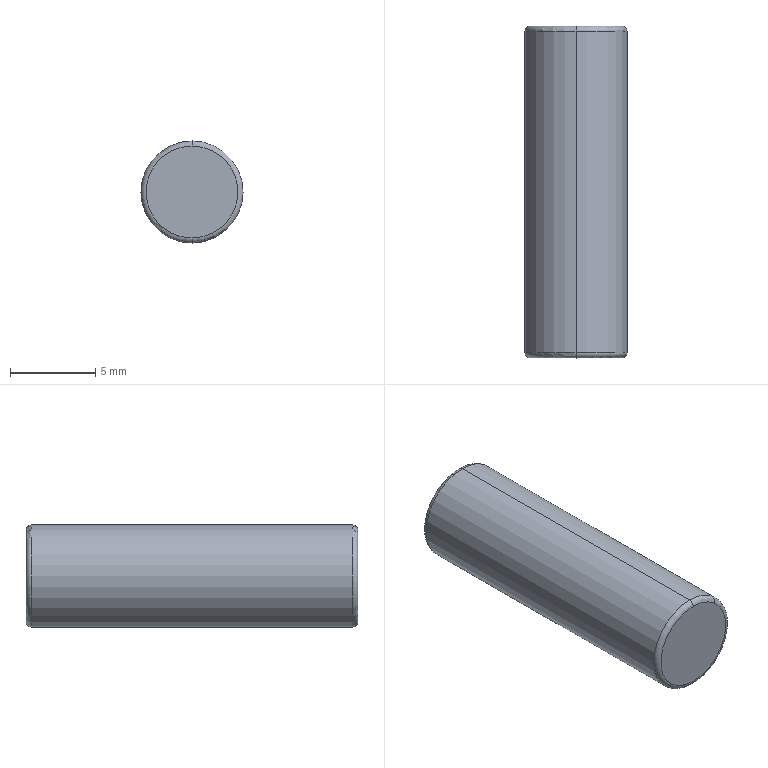Part | STEP file | 1 solid | 8 faces | box 6 x 19.5 x 6 mm | volume 550.638 mm3 | torus 4 | cylinder 2 | plane 2 | commonest cylinder face diameters 6 x2
STEP:
#1=CARTESIAN_POINT('',(0.,0.,0.));
#2=DIRECTION('',(0.,0.,1.));
#3=DIRECTION('',(1.,0.,0.));
#4=AXIS2_PLACEMENT_3D('',#1,#2,#3);
#5=CARTESIAN_POINT('',(0.,9.45,-3.));
#6=VERTEX_POINT('',#5);
#7=CARTESIAN_POINT('',(0.,9.45,3.));
#8=VERTEX_POINT('',#7);
#9=CARTESIAN_POINT('',(0.,9.45,0.));
#10=DIRECTION('',(0.,-1.,0.));
#11=DIRECTION('',(0.,0.,1.));
#12=AXIS2_PLACEMENT_3D('',#9,#10,#11);
#13=CIRCLE('',#12,3.);
#14=CARTESIAN_POINT('',(0.,9.45,0.));
#15=DIRECTION('',(0.,1.,0.));
#16=DIRECTION('',(0.,0.,1.));
#17=AXIS2_PLACEMENT_3D('',#14,#15,#16);
#18=TOROIDAL_SURFACE('',#17,2.7,0.3);
#19=CARTESIAN_POINT('',(6.283,0.));
#20=DIRECTION('',(-1.,0.));
#21=VECTOR('',#20,1.);
#22=LINE('',#19,#21);
#23=(GEOMETRIC_REPRESENTATION_CONTEXT(2)PARAMETRIC_REPRESENTATION_CONTEXT()REPRESENTATION_CONTEXT('',''));
#24=DEFINITIONAL_REPRESENTATION('',(#22),#23);
#25=PCURVE('',#18,#24);
#26=CARTESIAN_POINT('',(0.,9.75,0.));
#27=DIRECTION('',(0.,-1.,0.));
#28=DIRECTION('',(0.,0.,-1.));
#29=AXIS2_PLACEMENT_3D('',#26,#27,#28);
#30=CYLINDRICAL_SURFACE('',#29,3.);
#31=CARTESIAN_POINT('',(-3.142,0.3));
#32=DIRECTION('',(1.,0.));
#33=VECTOR('',#32,1.);
#34=LINE('',#31,#33);
#35=(GEOMETRIC_REPRESENTATION_CONTEXT(2)PARAMETRIC_REPRESENTATION_CONTEXT()REPRESENTATION_CONTEXT('',''));
#36=DEFINITIONAL_REPRESENTATION('',(#34),#35);
#37=PCURVE('',#30,#36);
#38=SURFACE_CURVE('',#13,(#25,#37),.PCURVE_S1.);
#39=EDGE_CURVE('',#6,#8,#38,.T.);
#40=ORIENTED_EDGE('',*,*,#39,.F.);
#41=CARTESIAN_POINT('',(0.,9.75,-2.7));
#42=VERTEX_POINT('',#41);
#43=CARTESIAN_POINT('',(0.,9.45,-2.7));
#44=DIRECTION('',(1.,0.,0.));
#45=DIRECTION('',(0.,0.,-1.));
#46=AXIS2_PLACEMENT_3D('',#43,#44,#45);
#47=CIRCLE('',#46,0.3);
#48=CARTESIAN_POINT('',(3.142,0.));
#49=DIRECTION('',(0.,1.));
#50=VECTOR('',#49,1.);
#51=LINE('',#48,#50);
#52=(GEOMETRIC_REPRESENTATION_CONTEXT(2)PARAMETRIC_REPRESENTATION_CONTEXT()REPRESENTATION_CONTEXT('',''));
#53=DEFINITIONAL_REPRESENTATION('',(#51),#52);
#54=PCURVE('',#18,#53);
#55=CARTESIAN_POINT('',(0.,9.45,0.));
#56=DIRECTION('',(0.,1.,0.));
#57=DIRECTION('',(0.,0.,1.));
#58=AXIS2_PLACEMENT_3D('',#55,#56,#57);
#59=TOROIDAL_SURFACE('',#58,2.7,0.3);
#60=CARTESIAN_POINT('',(3.142,0.));
#61=DIRECTION('',(0.,1.));
#62=VECTOR('',#61,1.);
#63=LINE('',#60,#62);
#64=(GEOMETRIC_REPRESENTATION_CONTEXT(2)PARAMETRIC_REPRESENTATION_CONTEXT()REPRESENTATION_CONTEXT('',''));
#65=DEFINITIONAL_REPRESENTATION('',(#63),#64);
#66=PCURVE('',#59,#65);
#67=SURFACE_CURVE('',#47,(#54,#66),.PCURVE_S1.);
#68=EDGE_CURVE('',#6,#42,#67,.T.);
#69=ORIENTED_EDGE('',*,*,#68,.T.);
#70=CARTESIAN_POINT('',(0.,9.75,2.7));
#71=VERTEX_POINT('',#70);
#72=CARTESIAN_POINT('',(0.,9.75,0.));
#73=DIRECTION('',(0.,1.,0.));
#74=DIRECTION('',(0.,0.,1.));
#75=AXIS2_PLACEMENT_3D('',#72,#73,#74);
#76=CIRCLE('',#75,2.7);
#77=CARTESIAN_POINT('',(0.,1.571));
#78=DIRECTION('',(1.,0.));
#79=VECTOR('',#78,1.);
#80=LINE('',#77,#79);
#81=(GEOMETRIC_REPRESENTATION_CONTEXT(2)PARAMETRIC_REPRESENTATION_CONTEXT()REPRESENTATION_CONTEXT('',''));
#82=DEFINITIONAL_REPRESENTATION('',(#80),#81);
#83=PCURVE('',#18,#82);
#84=CARTESIAN_POINT('',(0.,9.75,0.));
#85=DIRECTION('',(0.,1.,0.));
#86=DIRECTION('',(0.,0.,1.));
#87=AXIS2_PLACEMENT_3D('',#84,#85,#86);
#88=PLANE('',#87);
#89=CARTESIAN_POINT('',(0.,0.));
#90=DIRECTION('',(1.,0.));
#91=AXIS2_PLACEMENT_2D('',#89,#90);
#92=CIRCLE('',#91,2.7);
#93=(GEOMETRIC_REPRESENTATION_CONTEXT(2)PARAMETRIC_REPRESENTATION_CONTEXT()REPRESENTATION_CONTEXT('',''));
#94=DEFINITIONAL_REPRESENTATION('',(#92),#93);
#95=PCURVE('',#88,#94);
#96=SURFACE_CURVE('',#76,(#83,#95),.PCURVE_S1.);
#97=EDGE_CURVE('',#71,#42,#96,.T.);
#98=ORIENTED_EDGE('',*,*,#97,.F.);
#99=CARTESIAN_POINT('',(0.,9.45,2.7));
#100=DIRECTION('',(-1.,0.,0.));
#101=DIRECTION('',(0.,0.,1.));
#102=AXIS2_PLACEMENT_3D('',#99,#100,#101);
#103=CIRCLE('',#102,0.3);
#104=CARTESIAN_POINT('',(0.,0.));
#105=DIRECTION('',(0.,1.));
#106=VECTOR('',#105,1.);
#107=LINE('',#104,#106);
#108=(GEOMETRIC_REPRESENTATION_CONTEXT(2)PARAMETRIC_REPRESENTATION_CONTEXT()REPRESENTATION_CONTEXT('',''));
#109=DEFINITIONAL_REPRESENTATION('',(#107),#108);
#110=PCURVE('',#18,#109);
#111=CARTESIAN_POINT('',(6.283,0.));
#112=DIRECTION('',(0.,1.));
#113=VECTOR('',#112,1.);
#114=LINE('',#111,#113);
#115=(GEOMETRIC_REPRESENTATION_CONTEXT(2)PARAMETRIC_REPRESENTATION_CONTEXT()REPRESENTATION_CONTEXT('',''));
#116=DEFINITIONAL_REPRESENTATION('',(#114),#115);
#117=PCURVE('',#59,#116);
#118=SURFACE_CURVE('',#103,(#110,#117),.PCURVE_S1.);
#119=EDGE_CURVE('',#8,#71,#118,.T.);
#120=ORIENTED_EDGE('',*,*,#119,.F.);
#121=EDGE_LOOP('',(#40,#69,#98,#120));
#122=FACE_BOUND('',#121,.T.);
#123=ADVANCED_FACE('',(#122),#18,.T.);
#124=CARTESIAN_POINT('',(0.,-9.75,-2.7));
#125=VERTEX_POINT('',#124);
#126=CARTESIAN_POINT('',(0.,-9.75,2.7));
#127=VERTEX_POINT('',#126);
#128=CARTESIAN_POINT('',(0.,-9.75,0.));
#129=DIRECTION('',(0.,-1.,0.));
#130=DIRECTION('',(0.,0.,1.));
#131=AXIS2_PLACEMENT_3D('',#128,#129,#130);
#132=CIRCLE('',#131,2.7);
#133=CARTESIAN_POINT('',(0.,-9.45,0.));
#134=DIRECTION('',(0.,1.,0.));
#135=DIRECTION('',(0.,0.,1.));
#136=AXIS2_PLACEMENT_3D('',#133,#134,#135);
#137=TOROIDAL_SURFACE('',#136,2.7,0.3);
#138=CARTESIAN_POINT('',(6.283,4.712));
#139=DIRECTION('',(-1.,0.));
#140=VECTOR('',#139,1.);
#141=LINE('',#138,#140);
#142=(GEOMETRIC_REPRESENTATION_CONTEXT(2)PARAMETRIC_REPRESENTATION_CONTEXT()REPRESENTATION_CONTEXT('',''));
#143=DEFINITIONAL_REPRESENTATION('',(#141),#142);
#144=PCURVE('',#137,#143);
#145=CARTESIAN_POINT('',(0.,-9.75,0.));
#146=DIRECTION('',(0.,1.,0.));
#147=DIRECTION('',(0.,0.,1.));
#148=AXIS2_PLACEMENT_3D('',#145,#146,#147);
#149=PLANE('',#148);
#150=CARTESIAN_POINT('',(2.7,0.));
#151=CARTESIAN_POINT('',(2.7,-4.677));
#152=CARTESIAN_POINT('',(-1.35,-2.338));
#153=CARTESIAN_POINT('',(-5.4,0.));
#154=CARTESIAN_POINT('',(-1.35,2.338));
#155=CARTESIAN_POINT('',(2.7,4.677));
#156=CARTESIAN_POINT('',(2.7,0.));
#157=(BOUNDED_CURVE()B_SPLINE_CURVE(2,(#150,#151,#152,#153,#154,#155,#156),.UNSPECIFIED.,.T.,.F.)B_SPLINE_CURVE_WITH_KNOTS((1,2,2,2,2,1),(-2.094,0.,2.094,4.189,6.283,8.378),.UNSPECIFIED.)CURVE()GEOMETRIC_REPRESENTATION_ITEM()RATIONAL_B_SPLINE_CURVE((1.,0.5,1.,0.5,1.,0.5,1.))REPRESENTATION_ITEM(''));
#158=(GEOMETRIC_REPRESENTATION_CONTEXT(2)PARAMETRIC_REPRESENTATION_CONTEXT()REPRESENTATION_CONTEXT('',''));
#159=DEFINITIONAL_REPRESENTATION('',(#157),#158);
#160=PCURVE('',#149,#159);
#161=SURFACE_CURVE('',#132,(#144,#160),.PCURVE_S1.);
#162=EDGE_CURVE('',#125,#127,#161,.T.);
#163=ORIENTED_EDGE('',*,*,#162,.F.);
#164=CARTESIAN_POINT('',(0.,-9.45,-3.));
#165=VERTEX_POINT('',#164);
#166=CARTESIAN_POINT('',(0.,-9.45,-2.7));
#167=DIRECTION('',(1.,0.,0.));
#168=DIRECTION('',(0.,0.,-1.));
#169=AXIS2_PLACEMENT_3D('',#166,#167,#168);
#170=CIRCLE('',#169,0.3);
#171=CARTESIAN_POINT('',(3.142,0.));
#172=DIRECTION('',(0.,1.));
#173=VECTOR('',#172,1.);
#174=LINE('',#171,#173);
#175=(GEOMETRIC_REPRESENTATION_CONTEXT(2)PARAMETRIC_REPRESENTATION_CONTEXT()REPRESENTATION_CONTEXT('',''));
#176=DEFINITIONAL_REPRESENTATION('',(#174),#175);
#177=PCURVE('',#137,#176);
#178=CARTESIAN_POINT('',(0.,-9.45,0.));
#179=DIRECTION('',(0.,1.,0.));
#180=DIRECTION('',(0.,0.,1.));
#181=AXIS2_PLACEMENT_3D('',#178,#179,#180);
#182=TOROIDAL_SURFACE('',#181,2.7,0.3);
#183=CARTESIAN_POINT('',(3.142,0.));
#184=DIRECTION('',(0.,1.));
#185=VECTOR('',#184,1.);
#186=LINE('',#183,#185);
#187=(GEOMETRIC_REPRESENTATION_CONTEXT(2)PARAMETRIC_REPRESENTATION_CONTEXT()REPRESENTATION_CONTEXT('',''));
#188=DEFINITIONAL_REPRESENTATION('',(#186),#187);
#189=PCURVE('',#182,#188);
#190=SURFACE_CURVE('',#170,(#177,#189),.PCURVE_S1.);
#191=EDGE_CURVE('',#125,#165,#190,.T.);
#192=ORIENTED_EDGE('',*,*,#191,.T.);
#193=CARTESIAN_POINT('',(0.,-9.45,3.));
#194=VERTEX_POINT('',#193);
#195=CARTESIAN_POINT('',(0.,-9.45,0.));
#196=DIRECTION('',(0.,1.,0.));
#197=DIRECTION('',(0.,0.,1.));
#198=AXIS2_PLACEMENT_3D('',#195,#196,#197);
#199=CIRCLE('',#198,3.);
#200=CARTESIAN_POINT('',(0.,6.283));
#201=DIRECTION('',(1.,0.));
#202=VECTOR('',#201,1.);
#203=LINE('',#200,#202);
#204=(GEOMETRIC_REPRESENTATION_CONTEXT(2)PARAMETRIC_REPRESENTATION_CONTEXT()REPRESENTATION_CONTEXT('',''));
#205=DEFINITIONAL_REPRESENTATION('',(#203),#204);
#206=PCURVE('',#137,#205);
#207=CARTESIAN_POINT('',(3.142,19.2));
#208=DIRECTION('',(-1.,0.));
#209=VECTOR('',#208,1.);
#210=LINE('',#207,#209);
#211=(GEOMETRIC_REPRESENTATION_CONTEXT(2)PARAMETRIC_REPRESENTATION_CONTEXT()REPRESENTATION_CONTEXT('',''));
#212=DEFINITIONAL_REPRESENTATION('',(#210),#211);
#213=PCURVE('',#30,#212);
#214=SURFACE_CURVE('',#199,(#206,#213),.PCURVE_S1.);
#215=EDGE_CURVE('',#194,#165,#214,.T.);
#216=ORIENTED_EDGE('',*,*,#215,.F.);
#217=CARTESIAN_POINT('',(0.,-9.45,2.7));
#218=DIRECTION('',(-1.,0.,0.));
#219=DIRECTION('',(0.,0.,1.));
#220=AXIS2_PLACEMENT_3D('',#217,#218,#219);
#221=CIRCLE('',#220,0.3);
#222=CARTESIAN_POINT('',(0.,0.));
#223=DIRECTION('',(0.,1.));
#224=VECTOR('',#223,1.);
#225=LINE('',#222,#224);
#226=(GEOMETRIC_REPRESENTATION_CONTEXT(2)PARAMETRIC_REPRESENTATION_CONTEXT()REPRESENTATION_CONTEXT('',''));
#227=DEFINITIONAL_REPRESENTATION('',(#225),#226);
#228=PCURVE('',#137,#227);
#229=CARTESIAN_POINT('',(6.283,0.));
#230=DIRECTION('',(0.,1.));
#231=VECTOR('',#230,1.);
#232=LINE('',#229,#231);
#233=(GEOMETRIC_REPRESENTATION_CONTEXT(2)PARAMETRIC_REPRESENTATION_CONTEXT()REPRESENTATION_CONTEXT('',''));
#234=DEFINITIONAL_REPRESENTATION('',(#232),#233);
#235=PCURVE('',#182,#234);
#236=SURFACE_CURVE('',#221,(#228,#235),.PCURVE_S1.);
#237=EDGE_CURVE('',#127,#194,#236,.T.);
#238=ORIENTED_EDGE('',*,*,#237,.F.);
#239=EDGE_LOOP('',(#163,#192,#216,#238));
#240=FACE_BOUND('',#239,.T.);
#241=ADVANCED_FACE('',(#240),#137,.T.);
#242=ORIENTED_EDGE('',*,*,#39,.T.);
#243=CARTESIAN_POINT('',(0.,9.75,3.));
#244=DIRECTION('',(0.,-1.,0.));
#245=VECTOR('',#244,1.);
#246=LINE('',#243,#245);
#247=CARTESIAN_POINT('',(3.142,0.));
#248=DIRECTION('',(0.,1.));
#249=VECTOR('',#248,1.);
#250=LINE('',#247,#249);
#251=(GEOMETRIC_REPRESENTATION_CONTEXT(2)PARAMETRIC_REPRESENTATION_CONTEXT()REPRESENTATION_CONTEXT('',''));
#252=DEFINITIONAL_REPRESENTATION('',(#250),#251);
#253=PCURVE('',#30,#252);
#254=CARTESIAN_POINT('',(0.,9.75,0.));
#255=DIRECTION('',(0.,-1.,0.));
#256=DIRECTION('',(0.,0.,-1.));
#257=AXIS2_PLACEMENT_3D('',#254,#255,#256);
#258=CYLINDRICAL_SURFACE('',#257,3.);
#259=CARTESIAN_POINT('',(3.142,0.));
#260=DIRECTION('',(0.,1.));
#261=VECTOR('',#260,1.);
#262=LINE('',#259,#261);
#263=(GEOMETRIC_REPRESENTATION_CONTEXT(2)PARAMETRIC_REPRESENTATION_CONTEXT()REPRESENTATION_CONTEXT('',''));
#264=DEFINITIONAL_REPRESENTATION('',(#262),#263);
#265=PCURVE('',#258,#264);
#266=SURFACE_CURVE('',#246,(#253,#265),.PCURVE_S1.);
#267=EDGE_CURVE('',#8,#194,#266,.T.);
#268=ORIENTED_EDGE('',*,*,#267,.T.);
#269=ORIENTED_EDGE('',*,*,#215,.T.);
#270=CARTESIAN_POINT('',(0.,9.75,-3.));
#271=DIRECTION('',(0.,-1.,0.));
#272=VECTOR('',#271,1.);
#273=LINE('',#270,#272);
#274=CARTESIAN_POINT('',(0.,0.));
#275=DIRECTION('',(0.,1.));
#276=VECTOR('',#275,1.);
#277=LINE('',#274,#276);
#278=(GEOMETRIC_REPRESENTATION_CONTEXT(2)PARAMETRIC_REPRESENTATION_CONTEXT()REPRESENTATION_CONTEXT('',''));
#279=DEFINITIONAL_REPRESENTATION('',(#277),#278);
#280=PCURVE('',#30,#279);
#281=CARTESIAN_POINT('',(6.283,0.));
#282=DIRECTION('',(0.,1.));
#283=VECTOR('',#282,1.);
#284=LINE('',#281,#283);
#285=(GEOMETRIC_REPRESENTATION_CONTEXT(2)PARAMETRIC_REPRESENTATION_CONTEXT()REPRESENTATION_CONTEXT('',''));
#286=DEFINITIONAL_REPRESENTATION('',(#284),#285);
#287=PCURVE('',#258,#286);
#288=SURFACE_CURVE('',#273,(#280,#287),.PCURVE_S1.);
#289=EDGE_CURVE('',#6,#165,#288,.T.);
#290=ORIENTED_EDGE('',*,*,#289,.F.);
#291=EDGE_LOOP('',(#242,#268,#269,#290));
#292=FACE_BOUND('',#291,.T.);
#293=ADVANCED_FACE('',(#292),#30,.T.);
#294=ORIENTED_EDGE('',*,*,#267,.F.);
#295=CARTESIAN_POINT('',(0.,9.45,0.));
#296=DIRECTION('',(0.,-1.,0.));
#297=DIRECTION('',(0.,0.,1.));
#298=AXIS2_PLACEMENT_3D('',#295,#296,#297);
#299=CIRCLE('',#298,3.);
#300=CARTESIAN_POINT('',(3.142,0.3));
#301=DIRECTION('',(1.,0.));
#302=VECTOR('',#301,1.);
#303=LINE('',#300,#302);
#304=(GEOMETRIC_REPRESENTATION_CONTEXT(2)PARAMETRIC_REPRESENTATION_CONTEXT()REPRESENTATION_CONTEXT('',''));
#305=DEFINITIONAL_REPRESENTATION('',(#303),#304);
#306=PCURVE('',#258,#305);
#307=CARTESIAN_POINT('',(6.283,0.));
#308=DIRECTION('',(-1.,0.));
#309=VECTOR('',#308,1.);
#310=LINE('',#307,#309);
#311=(GEOMETRIC_REPRESENTATION_CONTEXT(2)PARAMETRIC_REPRESENTATION_CONTEXT()REPRESENTATION_CONTEXT('',''));
#312=DEFINITIONAL_REPRESENTATION('',(#310),#311);
#313=PCURVE('',#59,#312);
#314=SURFACE_CURVE('',#299,(#306,#313),.PCURVE_S1.);
#315=EDGE_CURVE('',#8,#6,#314,.T.);
#316=ORIENTED_EDGE('',*,*,#315,.T.);
#317=ORIENTED_EDGE('',*,*,#289,.T.);
#318=CARTESIAN_POINT('',(0.,-9.45,0.));
#319=DIRECTION('',(0.,1.,0.));
#320=DIRECTION('',(0.,0.,1.));
#321=AXIS2_PLACEMENT_3D('',#318,#319,#320);
#322=CIRCLE('',#321,3.);
#323=CARTESIAN_POINT('',(9.425,19.2));
#324=DIRECTION('',(-1.,0.));
#325=VECTOR('',#324,1.);
#326=LINE('',#323,#325);
#327=(GEOMETRIC_REPRESENTATION_CONTEXT(2)PARAMETRIC_REPRESENTATION_CONTEXT()REPRESENTATION_CONTEXT('',''));
#328=DEFINITIONAL_REPRESENTATION('',(#326),#327);
#329=PCURVE('',#258,#328);
#330=CARTESIAN_POINT('',(0.,6.283));
#331=DIRECTION('',(1.,0.));
#332=VECTOR('',#331,1.);
#333=LINE('',#330,#332);
#334=(GEOMETRIC_REPRESENTATION_CONTEXT(2)PARAMETRIC_REPRESENTATION_CONTEXT()REPRESENTATION_CONTEXT('',''));
#335=DEFINITIONAL_REPRESENTATION('',(#333),#334);
#336=PCURVE('',#182,#335);
#337=SURFACE_CURVE('',#322,(#329,#336),.PCURVE_S1.);
#338=EDGE_CURVE('',#165,#194,#337,.T.);
#339=ORIENTED_EDGE('',*,*,#338,.T.);
#340=EDGE_LOOP('',(#294,#316,#317,#339));
#341=FACE_BOUND('',#340,.T.);
#342=ADVANCED_FACE('',(#341),#258,.T.);
#343=ORIENTED_EDGE('',*,*,#97,.T.);
#344=CARTESIAN_POINT('',(0.,9.75,0.));
#345=DIRECTION('',(0.,1.,0.));
#346=DIRECTION('',(0.,0.,1.));
#347=AXIS2_PLACEMENT_3D('',#344,#345,#346);
#348=CIRCLE('',#347,2.7);
#349=CARTESIAN_POINT('',(0.,0.));
#350=DIRECTION('',(1.,0.));
#351=AXIS2_PLACEMENT_2D('',#349,#350);
#352=CIRCLE('',#351,2.7);
#353=(GEOMETRIC_REPRESENTATION_CONTEXT(2)PARAMETRIC_REPRESENTATION_CONTEXT()REPRESENTATION_CONTEXT('',''));
#354=DEFINITIONAL_REPRESENTATION('',(#352),#353);
#355=PCURVE('',#88,#354);
#356=CARTESIAN_POINT('',(0.,1.571));
#357=DIRECTION('',(1.,0.));
#358=VECTOR('',#357,1.);
#359=LINE('',#356,#358);
#360=(GEOMETRIC_REPRESENTATION_CONTEXT(2)PARAMETRIC_REPRESENTATION_CONTEXT()REPRESENTATION_CONTEXT('',''));
#361=DEFINITIONAL_REPRESENTATION('',(#359),#360);
#362=PCURVE('',#59,#361);
#363=SURFACE_CURVE('',#348,(#355,#362),.PCURVE_S1.);
#364=EDGE_CURVE('',#42,#71,#363,.T.);
#365=ORIENTED_EDGE('',*,*,#364,.T.);
#366=EDGE_LOOP('',(#343,#365));
#367=FACE_BOUND('',#366,.T.);
#368=ADVANCED_FACE('',(#367),#88,.T.);
#369=CARTESIAN_POINT('',(0.,-9.75,0.));
#370=DIRECTION('',(0.,-1.,0.));
#371=DIRECTION('',(0.,0.,1.));
#372=AXIS2_PLACEMENT_3D('',#369,#370,#371);
#373=CIRCLE('',#372,2.7);
#374=CARTESIAN_POINT('',(2.7,0.));
#375=CARTESIAN_POINT('',(2.7,-4.677));
#376=CARTESIAN_POINT('',(-1.35,-2.338));
#377=CARTESIAN_POINT('',(-5.4,0.));
#378=CARTESIAN_POINT('',(-1.35,2.338));
#379=CARTESIAN_POINT('',(2.7,4.677));
#380=CARTESIAN_POINT('',(2.7,0.));
#381=(BOUNDED_CURVE()B_SPLINE_CURVE(2,(#374,#375,#376,#377,#378,#379,#380),.UNSPECIFIED.,.T.,.F.)B_SPLINE_CURVE_WITH_KNOTS((1,2,2,2,2,1),(-2.094,0.,2.094,4.189,6.283,8.378),.UNSPECIFIED.)CURVE()GEOMETRIC_REPRESENTATION_ITEM()RATIONAL_B_SPLINE_CURVE((1.,0.5,1.,0.5,1.,0.5,1.))REPRESENTATION_ITEM(''));
#382=(GEOMETRIC_REPRESENTATION_CONTEXT(2)PARAMETRIC_REPRESENTATION_CONTEXT()REPRESENTATION_CONTEXT('',''));
#383=DEFINITIONAL_REPRESENTATION('',(#381),#382);
#384=PCURVE('',#149,#383);
#385=CARTESIAN_POINT('',(6.283,4.712));
#386=DIRECTION('',(-1.,0.));
#387=VECTOR('',#386,1.);
#388=LINE('',#385,#387);
#389=(GEOMETRIC_REPRESENTATION_CONTEXT(2)PARAMETRIC_REPRESENTATION_CONTEXT()REPRESENTATION_CONTEXT('',''));
#390=DEFINITIONAL_REPRESENTATION('',(#388),#389);
#391=PCURVE('',#182,#390);
#392=SURFACE_CURVE('',#373,(#384,#391),.PCURVE_S1.);
#393=EDGE_CURVE('',#127,#125,#392,.T.);
#394=ORIENTED_EDGE('',*,*,#393,.T.);
#395=ORIENTED_EDGE('',*,*,#162,.T.);
#396=EDGE_LOOP('',(#394,#395));
#397=FACE_BOUND('',#396,.T.);
#398=ADVANCED_FACE('',(#397),#149,.F.);
#399=ORIENTED_EDGE('',*,*,#191,.F.);
#400=ORIENTED_EDGE('',*,*,#393,.F.);
#401=ORIENTED_EDGE('',*,*,#237,.T.);
#402=ORIENTED_EDGE('',*,*,#338,.F.);
#403=EDGE_LOOP('',(#399,#400,#401,#402));
#404=FACE_BOUND('',#403,.T.);
#405=ADVANCED_FACE('',(#404),#182,.T.);
#406=ORIENTED_EDGE('',*,*,#68,.F.);
#407=ORIENTED_EDGE('',*,*,#315,.F.);
#408=ORIENTED_EDGE('',*,*,#119,.T.);
#409=ORIENTED_EDGE('',*,*,#364,.F.);
#410=EDGE_LOOP('',(#406,#407,#408,#409));
#411=FACE_BOUND('',#410,.T.);
#412=ADVANCED_FACE('',(#411),#59,.T.);
#413=CLOSED_SHELL('',(#123,#241,#293,#342,#368,#398,#405,#412));
#414=MANIFOLD_SOLID_BREP('',#413);
#415=(LENGTH_UNIT()NAMED_UNIT(*)SI_UNIT(.MILLI.,.METRE.));
#416=UNCERTAINTY_MEASURE_WITH_UNIT(LENGTH_MEASURE(0.0000001),#415,'','');
#417=(NAMED_UNIT(*)PLANE_ANGLE_UNIT()SI_UNIT($,.RADIAN.));
#418=(NAMED_UNIT(*)SI_UNIT($,.STERADIAN.)SOLID_ANGLE_UNIT());
#419=(GEOMETRIC_REPRESENTATION_CONTEXT(3)GLOBAL_UNCERTAINTY_ASSIGNED_CONTEXT((#416))GLOBAL_UNIT_ASSIGNED_CONTEXT((#415,#417,#418))REPRESENTATION_CONTEXT('',''));
#420=ADVANCED_BREP_SHAPE_REPRESENTATION('',(#4,#414),#419);